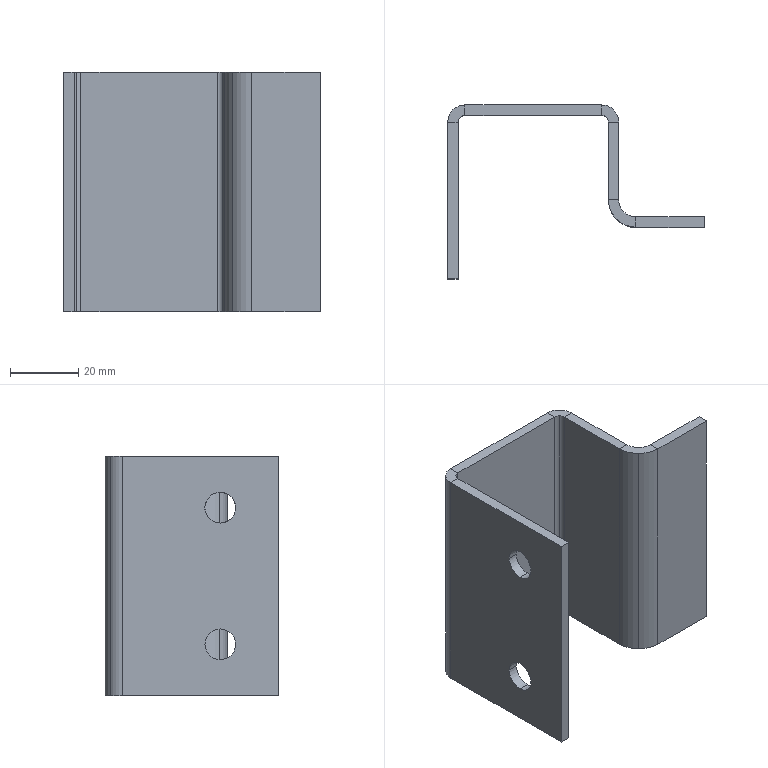Part | NX | features BREP 1 | 1 solid | 44 faces | box 75 x 50.821 x 70 mm | volume 31072 mm3 | plane 24 | cylinder 20 | commonest cylinder face diameters 9 x8 10 x6 4 x4 16 x2
STEP:
#1=CARTESIAN_POINT('',(1716.53,-660.002,420.012));
#2=VERTEX_POINT('',#1);
#3=CARTESIAN_POINT('',(1716.53,-660.002,490.012));
#4=VERTEX_POINT('',#3);
#5=CARTESIAN_POINT('',(1716.53,-660.002,455.012));
#6=DIRECTION('',(0.,0.,1.));
#7=VECTOR('',#6,1000.);
#8=LINE('',#5,#7);
#9=EDGE_CURVE('',#2,#4,#8,.T.);
#10=ORIENTED_EDGE('',*,*,#9,.T.);
#11=CARTESIAN_POINT('',(1696.53,-660.002,490.012));
#12=VERTEX_POINT('',#11);
#13=CARTESIAN_POINT('',(1706.53,-660.002,490.012));
#14=DIRECTION('',(1.,0.,0.));
#15=VECTOR('',#14,1000.);
#16=LINE('',#13,#15);
#17=EDGE_CURVE('',#12,#4,#16,.T.);
#18=ORIENTED_EDGE('',*,*,#17,.F.);
#19=CARTESIAN_POINT('',(1696.53,-660.002,420.012));
#20=VERTEX_POINT('',#19);
#21=CARTESIAN_POINT('',(1696.53,-660.002,455.012));
#22=DIRECTION('',(0.,0.,1.));
#23=VECTOR('',#22,1000.);
#24=LINE('',#21,#23);
#25=EDGE_CURVE('',#20,#12,#24,.T.);
#26=ORIENTED_EDGE('',*,*,#25,.F.);
#27=CARTESIAN_POINT('',(1706.53,-660.002,420.012));
#28=DIRECTION('',(1.,0.,0.));
#29=VECTOR('',#28,1000.);
#30=LINE('',#27,#29);
#31=EDGE_CURVE('',#20,#2,#30,.T.);
#32=ORIENTED_EDGE('',*,*,#31,.T.);
#33=EDGE_LOOP('',(#10,#18,#26,#32));
#34=FACE_BOUND('',#33,.T.);
#35=CARTESIAN_POINT('',(1691.53,-660.002,455.012));
#36=DIRECTION('',(0.,-1.,0.));
#37=DIRECTION('',(1.,0.,0.));
#38=AXIS2_PLACEMENT_3D('',#35,#36,#37);
#39=PLANE('',#38);
#40=ADVANCED_FACE('',(#34),#39,.T.);
#41=CARTESIAN_POINT('',(1696.53,-657.002,420.012));
#42=VERTEX_POINT('',#41);
#43=CARTESIAN_POINT('',(1716.53,-657.002,420.012));
#44=VERTEX_POINT('',#43);
#45=CARTESIAN_POINT('',(1706.53,-657.002,420.012));
#46=DIRECTION('',(1.,0.,0.));
#47=VECTOR('',#46,1000.);
#48=LINE('',#45,#47);
#49=EDGE_CURVE('',#42,#44,#48,.T.);
#50=ORIENTED_EDGE('',*,*,#49,.F.);
#51=CARTESIAN_POINT('',(1696.53,-657.002,490.012));
#52=VERTEX_POINT('',#51);
#53=CARTESIAN_POINT('',(1696.53,-657.002,455.012));
#54=DIRECTION('',(0.,0.,1.));
#55=VECTOR('',#54,1000.);
#56=LINE('',#53,#55);
#57=EDGE_CURVE('',#42,#52,#56,.T.);
#58=ORIENTED_EDGE('',*,*,#57,.T.);
#59=CARTESIAN_POINT('',(1716.53,-657.002,490.012));
#60=VERTEX_POINT('',#59);
#61=CARTESIAN_POINT('',(1706.53,-657.002,490.012));
#62=DIRECTION('',(1.,0.,0.));
#63=VECTOR('',#62,1000.);
#64=LINE('',#61,#63);
#65=EDGE_CURVE('',#52,#60,#64,.T.);
#66=ORIENTED_EDGE('',*,*,#65,.T.);
#67=CARTESIAN_POINT('',(1716.53,-657.002,455.012));
#68=DIRECTION('',(0.,0.,1.));
#69=VECTOR('',#68,1000.);
#70=LINE('',#67,#69);
#71=EDGE_CURVE('',#44,#60,#70,.T.);
#72=ORIENTED_EDGE('',*,*,#71,.F.);
#73=EDGE_LOOP('',(#50,#58,#66,#72));
#74=FACE_BOUND('',#73,.T.);
#75=CARTESIAN_POINT('',(1691.53,-657.002,455.012));
#76=DIRECTION('',(0.,-1.,0.));
#77=DIRECTION('',(1.,0.,0.));
#78=AXIS2_PLACEMENT_3D('',#75,#76,#77);
#79=PLANE('',#78);
#80=ADVANCED_FACE('',(#74),#79,.F.);
#81=ORIENTED_EDGE('',*,*,#9,.F.);
#82=CARTESIAN_POINT('',(1716.53,-658.502,420.012));
#83=DIRECTION('',(0.,1.,0.));
#84=VECTOR('',#83,1000.);
#85=LINE('',#82,#84);
#86=EDGE_CURVE('',#2,#44,#85,.T.);
#87=ORIENTED_EDGE('',*,*,#86,.T.);
#88=ORIENTED_EDGE('',*,*,#71,.T.);
#89=CARTESIAN_POINT('',(1716.53,-658.502,490.012));
#90=DIRECTION('',(0.,1.,0.));
#91=VECTOR('',#90,1000.);
#92=LINE('',#89,#91);
#93=EDGE_CURVE('',#4,#60,#92,.T.);
#94=ORIENTED_EDGE('',*,*,#93,.F.);
#95=EDGE_LOOP('',(#81,#87,#88,#94));
#96=FACE_BOUND('',#95,.T.);
#97=CARTESIAN_POINT('',(1716.53,-660.002,455.012));
#98=DIRECTION('',(1.,0.,0.));
#99=DIRECTION('',(0.,1.,0.));
#100=AXIS2_PLACEMENT_3D('',#97,#98,#99);
#101=PLANE('',#100);
#102=ADVANCED_FACE('',(#96),#101,.T.);
#103=ORIENTED_EDGE('',*,*,#31,.F.);
#104=CARTESIAN_POINT('',(1696.53,-658.502,420.012));
#105=DIRECTION('',(0.,-1.,0.));
#106=VECTOR('',#105,1000.);
#107=LINE('',#104,#106);
#108=EDGE_CURVE('',#42,#20,#107,.T.);
#109=ORIENTED_EDGE('',*,*,#108,.F.);
#110=ORIENTED_EDGE('',*,*,#49,.T.);
#111=ORIENTED_EDGE('',*,*,#86,.F.);
#112=EDGE_LOOP('',(#103,#109,#110,#111));
#113=FACE_BOUND('',#112,.T.);
#114=CARTESIAN_POINT('',(1706.53,-660.002,420.012));
#115=DIRECTION('',(0.,0.,1.));
#116=DIRECTION('',(1.,0.,0.));
#117=AXIS2_PLACEMENT_3D('',#114,#115,#116);
#118=PLANE('',#117);
#119=ADVANCED_FACE('',(#113),#118,.F.);
#120=CARTESIAN_POINT('',(1690.873,-657.658,420.012));
#121=VERTEX_POINT('',#120);
#122=CARTESIAN_POINT('',(1690.873,-657.658,490.012));
#123=VERTEX_POINT('',#122);
#124=CARTESIAN_POINT('',(1690.873,-657.658,455.012));
#125=DIRECTION('',(0.,0.,1.));
#126=VECTOR('',#125,1000.);
#127=LINE('',#124,#126);
#128=EDGE_CURVE('',#121,#123,#127,.T.);
#129=ORIENTED_EDGE('',*,*,#128,.F.);
#130=CARTESIAN_POINT('',(1696.53,-652.002,420.012));
#131=DIRECTION('',(0.,0.,1.));
#132=DIRECTION('',(1.,0.,0.));
#133=AXIS2_PLACEMENT_3D('',#130,#131,#132);
#134=CIRCLE('',#133,8.);
#135=EDGE_CURVE('',#121,#20,#134,.T.);
#136=ORIENTED_EDGE('',*,*,#135,.T.);
#137=ORIENTED_EDGE('',*,*,#25,.T.);
#138=CARTESIAN_POINT('',(1696.53,-652.002,490.012));
#139=DIRECTION('',(0.,0.,1.));
#140=DIRECTION('',(1.,0.,0.));
#141=AXIS2_PLACEMENT_3D('',#138,#139,#140);
#142=CIRCLE('',#141,8.);
#143=EDGE_CURVE('',#123,#12,#142,.T.);
#144=ORIENTED_EDGE('',*,*,#143,.F.);
#145=EDGE_LOOP('',(#129,#136,#137,#144));
#146=FACE_BOUND('',#145,.T.);
#147=CARTESIAN_POINT('',(1696.53,-652.002,455.012));
#148=DIRECTION('',(0.,0.,1.));
#149=DIRECTION('',(-0.7071,-0.7071,0.));
#150=AXIS2_PLACEMENT_3D('',#147,#148,#149);
#151=CYLINDRICAL_SURFACE('',#150,8.);
#152=ADVANCED_FACE('',(#146),#151,.T.);
#153=CARTESIAN_POINT('',(1691.53,-652.002,420.012));
#154=VERTEX_POINT('',#153);
#155=CARTESIAN_POINT('',(1692.995,-655.537,420.012));
#156=VERTEX_POINT('',#155);
#157=CARTESIAN_POINT('',(1696.53,-652.002,420.012));
#158=DIRECTION('',(0.,0.,1.));
#159=DIRECTION('',(1.,0.,0.));
#160=AXIS2_PLACEMENT_3D('',#157,#158,#159);
#161=CIRCLE('',#160,5.);
#162=EDGE_CURVE('',#154,#156,#161,.T.);
#163=ORIENTED_EDGE('',*,*,#162,.F.);
#164=CARTESIAN_POINT('',(1691.53,-652.002,490.012));
#165=VERTEX_POINT('',#164);
#166=CARTESIAN_POINT('',(1691.53,-652.002,455.012));
#167=DIRECTION('',(0.,0.,1.));
#168=VECTOR('',#167,1000.);
#169=LINE('',#166,#168);
#170=EDGE_CURVE('',#154,#165,#169,.T.);
#171=ORIENTED_EDGE('',*,*,#170,.T.);
#172=CARTESIAN_POINT('',(1692.995,-655.537,490.012));
#173=VERTEX_POINT('',#172);
#174=CARTESIAN_POINT('',(1696.53,-652.002,490.012));
#175=DIRECTION('',(0.,0.,1.));
#176=DIRECTION('',(1.,0.,0.));
#177=AXIS2_PLACEMENT_3D('',#174,#175,#176);
#178=CIRCLE('',#177,5.);
#179=EDGE_CURVE('',#165,#173,#178,.T.);
#180=ORIENTED_EDGE('',*,*,#179,.T.);
#181=CARTESIAN_POINT('',(1692.995,-655.537,455.012));
#182=DIRECTION('',(0.,0.,1.));
#183=VECTOR('',#182,1000.);
#184=LINE('',#181,#183);
#185=EDGE_CURVE('',#156,#173,#184,.T.);
#186=ORIENTED_EDGE('',*,*,#185,.F.);
#187=EDGE_LOOP('',(#163,#171,#180,#186));
#188=FACE_BOUND('',#187,.T.);
#189=CARTESIAN_POINT('',(1696.53,-652.002,455.012));
#190=DIRECTION('',(0.,0.,1.));
#191=DIRECTION('',(0.7071,0.7071,0.));
#192=AXIS2_PLACEMENT_3D('',#189,#190,#191);
#193=CYLINDRICAL_SURFACE('',#192,5.);
#194=ADVANCED_FACE('',(#188),#193,.F.);
#195=CARTESIAN_POINT('',(1696.53,-652.002,490.012));
#196=DIRECTION('',(0.,0.,1.));
#197=DIRECTION('',(1.,0.,0.));
#198=AXIS2_PLACEMENT_3D('',#195,#196,#197);
#199=CIRCLE('',#198,5.);
#200=EDGE_CURVE('',#173,#52,#199,.T.);
#201=ORIENTED_EDGE('',*,*,#200,.T.);
#202=ORIENTED_EDGE('',*,*,#57,.F.);
#203=CARTESIAN_POINT('',(1696.53,-652.002,420.012));
#204=DIRECTION('',(0.,0.,1.));
#205=DIRECTION('',(1.,0.,0.));
#206=AXIS2_PLACEMENT_3D('',#203,#204,#205);
#207=CIRCLE('',#206,5.);
#208=EDGE_CURVE('',#156,#42,#207,.T.);
#209=ORIENTED_EDGE('',*,*,#208,.F.);
#210=ORIENTED_EDGE('',*,*,#185,.T.);
#211=EDGE_LOOP('',(#201,#202,#209,#210));
#212=FACE_BOUND('',#211,.T.);
#213=CARTESIAN_POINT('',(1696.53,-652.002,455.012));
#214=DIRECTION('',(0.,0.,1.));
#215=DIRECTION('',(-0.7071,-0.7071,0.));
#216=AXIS2_PLACEMENT_3D('',#213,#214,#215);
#217=CYLINDRICAL_SURFACE('',#216,5.);
#218=ADVANCED_FACE('',(#212),#217,.F.);
#219=ORIENTED_EDGE('',*,*,#93,.T.);
#220=ORIENTED_EDGE('',*,*,#65,.F.);
#221=CARTESIAN_POINT('',(1696.53,-658.502,490.012));
#222=DIRECTION('',(0.,-1.,0.));
#223=VECTOR('',#222,1000.);
#224=LINE('',#221,#223);
#225=EDGE_CURVE('',#52,#12,#224,.T.);
#226=ORIENTED_EDGE('',*,*,#225,.T.);
#227=ORIENTED_EDGE('',*,*,#17,.T.);
#228=EDGE_LOOP('',(#219,#220,#226,#227));
#229=FACE_BOUND('',#228,.T.);
#230=CARTESIAN_POINT('',(1706.53,-660.002,490.012));
#231=DIRECTION('',(0.,0.,1.));
#232=DIRECTION('',(1.,0.,0.));
#233=AXIS2_PLACEMENT_3D('',#230,#231,#232);
#234=PLANE('',#233);
#235=ADVANCED_FACE('',(#229),#234,.T.);
#236=ORIENTED_EDGE('',*,*,#128,.T.);
#237=CARTESIAN_POINT('',(1688.53,-652.002,490.012));
#238=VERTEX_POINT('',#237);
#239=CARTESIAN_POINT('',(1696.53,-652.002,490.012));
#240=DIRECTION('',(0.,0.,1.));
#241=DIRECTION('',(1.,0.,0.));
#242=AXIS2_PLACEMENT_3D('',#239,#240,#241);
#243=CIRCLE('',#242,8.);
#244=EDGE_CURVE('',#238,#123,#243,.T.);
#245=ORIENTED_EDGE('',*,*,#244,.F.);
#246=CARTESIAN_POINT('',(1688.53,-652.002,420.012));
#247=VERTEX_POINT('',#246);
#248=CARTESIAN_POINT('',(1688.53,-652.002,455.012));
#249=DIRECTION('',(0.,0.,1.));
#250=VECTOR('',#249,1000.);
#251=LINE('',#248,#250);
#252=EDGE_CURVE('',#247,#238,#251,.T.);
#253=ORIENTED_EDGE('',*,*,#252,.F.);
#254=CARTESIAN_POINT('',(1696.53,-652.002,420.012));
#255=DIRECTION('',(0.,0.,1.));
#256=DIRECTION('',(1.,0.,0.));
#257=AXIS2_PLACEMENT_3D('',#254,#255,#256);
#258=CIRCLE('',#257,8.);
#259=EDGE_CURVE('',#247,#121,#258,.T.);
#260=ORIENTED_EDGE('',*,*,#259,.T.);
#261=EDGE_LOOP('',(#236,#245,#253,#260));
#262=FACE_BOUND('',#261,.T.);
#263=CARTESIAN_POINT('',(1696.53,-652.002,455.012));
#264=DIRECTION('',(0.,0.,1.));
#265=DIRECTION('',(0.7071,0.7071,0.));
#266=AXIS2_PLACEMENT_3D('',#263,#264,#265);
#267=CYLINDRICAL_SURFACE('',#266,8.);
#268=ADVANCED_FACE('',(#262),#267,.T.);
#269=ORIENTED_EDGE('',*,*,#135,.F.);
#270=ORIENTED_EDGE('',*,*,#259,.F.);
#271=CARTESIAN_POINT('',(1690.03,-652.002,420.012));
#272=DIRECTION('',(-1.,0.,0.));
#273=VECTOR('',#272,1000.);
#274=LINE('',#271,#273);
#275=EDGE_CURVE('',#154,#247,#274,.T.);
#276=ORIENTED_EDGE('',*,*,#275,.F.);
#277=ORIENTED_EDGE('',*,*,#162,.T.);
#278=ORIENTED_EDGE('',*,*,#208,.T.);
#279=ORIENTED_EDGE('',*,*,#108,.T.);
#280=EDGE_LOOP('',(#269,#270,#276,#277,#278,#279));
#281=FACE_BOUND('',#280,.T.);
#282=CARTESIAN_POINT('',(1688.53,-652.002,420.012));
#283=DIRECTION('',(0.,0.,1.));
#284=DIRECTION('',(0.3827,-0.9239,0.));
#285=AXIS2_PLACEMENT_3D('',#282,#283,#284);
#286=PLANE('',#285);
#287=ADVANCED_FACE('',(#281),#286,.F.);
#288=CARTESIAN_POINT('',(1691.53,-629.251,490.012));
#289=VERTEX_POINT('',#288);
#290=CARTESIAN_POINT('',(1691.53,-640.626,490.012));
#291=DIRECTION('',(0.,1.,0.));
#292=VECTOR('',#291,1000.);
#293=LINE('',#290,#292);
#294=EDGE_CURVE('',#165,#289,#293,.T.);
#295=ORIENTED_EDGE('',*,*,#294,.F.);
#296=ORIENTED_EDGE('',*,*,#170,.F.);
#297=CARTESIAN_POINT('',(1691.53,-629.251,420.012));
#298=VERTEX_POINT('',#297);
#299=CARTESIAN_POINT('',(1691.53,-640.626,420.012));
#300=DIRECTION('',(0.,-1.,0.));
#301=VECTOR('',#300,1000.);
#302=LINE('',#299,#301);
#303=EDGE_CURVE('',#298,#154,#302,.T.);
#304=ORIENTED_EDGE('',*,*,#303,.F.);
#305=CARTESIAN_POINT('',(1691.53,-629.251,455.012));
#306=DIRECTION('',(0.,0.,1.));
#307=VECTOR('',#306,1000.);
#308=LINE('',#305,#307);
#309=EDGE_CURVE('',#298,#289,#308,.T.);
#310=ORIENTED_EDGE('',*,*,#309,.T.);
#311=EDGE_LOOP('',(#295,#296,#304,#310));
#312=FACE_BOUND('',#311,.T.);
#313=CARTESIAN_POINT('',(1691.53,-624.251,455.012));
#314=DIRECTION('',(-1.,0.,0.));
#315=DIRECTION('',(0.,-1.,0.));
#316=AXIS2_PLACEMENT_3D('',#313,#314,#315);
#317=PLANE('',#316);
#318=ADVANCED_FACE('',(#312),#317,.F.);
#319=ORIENTED_EDGE('',*,*,#225,.F.);
#320=ORIENTED_EDGE('',*,*,#200,.F.);
#321=ORIENTED_EDGE('',*,*,#179,.F.);
#322=CARTESIAN_POINT('',(1690.03,-652.002,490.012));
#323=DIRECTION('',(-1.,0.,0.));
#324=VECTOR('',#323,1000.);
#325=LINE('',#322,#324);
#326=EDGE_CURVE('',#165,#238,#325,.T.);
#327=ORIENTED_EDGE('',*,*,#326,.T.);
#328=ORIENTED_EDGE('',*,*,#244,.T.);
#329=ORIENTED_EDGE('',*,*,#143,.T.);
#330=EDGE_LOOP('',(#319,#320,#321,#327,#328,#329));
#331=FACE_BOUND('',#330,.T.);
#332=CARTESIAN_POINT('',(1688.53,-652.002,490.012));
#333=DIRECTION('',(0.,0.,1.));
#334=DIRECTION('',(0.3827,-0.9239,0.));
#335=AXIS2_PLACEMENT_3D('',#332,#333,#334);
#336=PLANE('',#335);
#337=ADVANCED_FACE('',(#331),#336,.T.);
#338=CARTESIAN_POINT('',(1688.53,-629.251,420.012));
#339=VERTEX_POINT('',#338);
#340=CARTESIAN_POINT('',(1688.53,-629.251,490.012));
#341=VERTEX_POINT('',#340);
#342=CARTESIAN_POINT('',(1688.53,-629.251,455.012));
#343=DIRECTION('',(0.,0.,1.));
#344=VECTOR('',#343,1000.);
#345=LINE('',#342,#344);
#346=EDGE_CURVE('',#339,#341,#345,.T.);
#347=ORIENTED_EDGE('',*,*,#346,.F.);
#348=CARTESIAN_POINT('',(1688.53,-640.626,420.012));
#349=DIRECTION('',(0.,-1.,0.));
#350=VECTOR('',#349,1000.);
#351=LINE('',#348,#350);
#352=EDGE_CURVE('',#339,#247,#351,.T.);
#353=ORIENTED_EDGE('',*,*,#352,.T.);
#354=ORIENTED_EDGE('',*,*,#252,.T.);
#355=CARTESIAN_POINT('',(1688.53,-640.626,490.012));
#356=DIRECTION('',(0.,1.,0.));
#357=VECTOR('',#356,1000.);
#358=LINE('',#355,#357);
#359=EDGE_CURVE('',#238,#341,#358,.T.);
#360=ORIENTED_EDGE('',*,*,#359,.T.);
#361=EDGE_LOOP('',(#347,#353,#354,#360));
#362=FACE_BOUND('',#361,.T.);
#363=CARTESIAN_POINT('',(1688.53,-624.251,455.012));
#364=DIRECTION('',(-1.,0.,0.));
#365=DIRECTION('',(0.,-1.,0.));
#366=AXIS2_PLACEMENT_3D('',#363,#364,#365);
#367=PLANE('',#366);
#368=ADVANCED_FACE('',(#362),#367,.T.);
#369=CARTESIAN_POINT('',(1690.03,-629.251,420.012));
#370=DIRECTION('',(1.,0.,0.));
#371=VECTOR('',#370,1000.);
#372=LINE('',#369,#371);
#373=EDGE_CURVE('',#339,#298,#372,.T.);
#374=ORIENTED_EDGE('',*,*,#373,.T.);
#375=ORIENTED_EDGE('',*,*,#303,.T.);
#376=ORIENTED_EDGE('',*,*,#275,.T.);
#377=ORIENTED_EDGE('',*,*,#352,.F.);
#378=EDGE_LOOP('',(#374,#375,#376,#377));
#379=FACE_BOUND('',#378,.T.);
#380=CARTESIAN_POINT('',(1688.53,-640.626,420.012));
#381=DIRECTION('',(0.,0.,1.));
#382=DIRECTION('',(1.,0.,0.));
#383=AXIS2_PLACEMENT_3D('',#380,#381,#382);
#384=PLANE('',#383);
#385=ADVANCED_FACE('',(#379),#384,.F.);
#386=CARTESIAN_POINT('',(1690.066,-625.715,420.012));
#387=VERTEX_POINT('',#386);
#388=CARTESIAN_POINT('',(1690.066,-625.715,490.012));
#389=VERTEX_POINT('',#388);
#390=CARTESIAN_POINT('',(1690.066,-625.715,455.012));
#391=DIRECTION('',(0.,0.,1.));
#392=VECTOR('',#391,1000.);
#393=LINE('',#390,#392);
#394=EDGE_CURVE('',#387,#389,#393,.T.);
#395=ORIENTED_EDGE('',*,*,#394,.T.);
#396=CARTESIAN_POINT('',(1686.53,-629.251,490.012));
#397=DIRECTION('',(0.,0.,1.));
#398=DIRECTION('',(1.,0.,0.));
#399=AXIS2_PLACEMENT_3D('',#396,#397,#398);
#400=CIRCLE('',#399,5.);
#401=EDGE_CURVE('',#289,#389,#400,.T.);
#402=ORIENTED_EDGE('',*,*,#401,.F.);
#403=ORIENTED_EDGE('',*,*,#309,.F.);
#404=CARTESIAN_POINT('',(1686.53,-629.251,420.012));
#405=DIRECTION('',(0.,0.,1.));
#406=DIRECTION('',(1.,0.,0.));
#407=AXIS2_PLACEMENT_3D('',#404,#405,#406);
#408=CIRCLE('',#407,5.);
#409=EDGE_CURVE('',#298,#387,#408,.T.);
#410=ORIENTED_EDGE('',*,*,#409,.T.);
#411=EDGE_LOOP('',(#395,#402,#403,#410));
#412=FACE_BOUND('',#411,.T.);
#413=CARTESIAN_POINT('',(1686.53,-629.251,455.012));
#414=DIRECTION('',(0.,0.,1.));
#415=DIRECTION('',(-0.7071,-0.7071,0.));
#416=AXIS2_PLACEMENT_3D('',#413,#414,#415);
#417=CYLINDRICAL_SURFACE('',#416,5.);
#418=ADVANCED_FACE('',(#412),#417,.T.);
#419=ORIENTED_EDGE('',*,*,#359,.F.);
#420=ORIENTED_EDGE('',*,*,#326,.F.);
#421=ORIENTED_EDGE('',*,*,#294,.T.);
#422=CARTESIAN_POINT('',(1690.03,-629.251,490.012));
#423=DIRECTION('',(1.,0.,0.));
#424=VECTOR('',#423,1000.);
#425=LINE('',#422,#424);
#426=EDGE_CURVE('',#341,#289,#425,.T.);
#427=ORIENTED_EDGE('',*,*,#426,.F.);
#428=EDGE_LOOP('',(#419,#420,#421,#427));
#429=FACE_BOUND('',#428,.T.);
#430=CARTESIAN_POINT('',(1688.53,-640.626,490.012));
#431=DIRECTION('',(0.,0.,1.));
#432=DIRECTION('',(1.,0.,0.));
#433=AXIS2_PLACEMENT_3D('',#430,#431,#432);
#434=PLANE('',#433);
#435=ADVANCED_FACE('',(#429),#434,.T.);
#436=CARTESIAN_POINT('',(1687.944,-627.837,420.012));
#437=VERTEX_POINT('',#436);
#438=CARTESIAN_POINT('',(1686.53,-629.251,420.012));
#439=DIRECTION('',(0.,0.,1.));
#440=DIRECTION('',(1.,0.,0.));
#441=AXIS2_PLACEMENT_3D('',#438,#439,#440);
#442=CIRCLE('',#441,2.);
#443=EDGE_CURVE('',#339,#437,#442,.T.);
#444=ORIENTED_EDGE('',*,*,#443,.F.);
#445=ORIENTED_EDGE('',*,*,#346,.T.);
#446=CARTESIAN_POINT('',(1687.944,-627.837,490.012));
#447=VERTEX_POINT('',#446);
#448=CARTESIAN_POINT('',(1686.53,-629.251,490.012));
#449=DIRECTION('',(0.,0.,1.));
#450=DIRECTION('',(1.,0.,0.));
#451=AXIS2_PLACEMENT_3D('',#448,#449,#450);
#452=CIRCLE('',#451,2.);
#453=EDGE_CURVE('',#341,#447,#452,.T.);
#454=ORIENTED_EDGE('',*,*,#453,.T.);
#455=CARTESIAN_POINT('',(1687.944,-627.837,455.012));
#456=DIRECTION('',(0.,0.,1.));
#457=VECTOR('',#456,1000.);
#458=LINE('',#455,#457);
#459=EDGE_CURVE('',#437,#447,#458,.T.);
#460=ORIENTED_EDGE('',*,*,#459,.F.);
#461=EDGE_LOOP('',(#444,#445,#454,#460));
#462=FACE_BOUND('',#461,.T.);
#463=CARTESIAN_POINT('',(1686.53,-629.251,455.012));
#464=DIRECTION('',(0.,0.,1.));
#465=DIRECTION('',(-0.7071,-0.7071,0.));
#466=AXIS2_PLACEMENT_3D('',#463,#464,#465);
#467=CYLINDRICAL_SURFACE('',#466,2.);
#468=ADVANCED_FACE('',(#462),#467,.F.);
#469=CARTESIAN_POINT('',(1686.53,-627.251,490.012));
#470=VERTEX_POINT('',#469);
#471=CARTESIAN_POINT('',(1686.53,-629.251,490.012));
#472=DIRECTION('',(0.,0.,1.));
#473=DIRECTION('',(1.,0.,0.));
#474=AXIS2_PLACEMENT_3D('',#471,#472,#473);
#475=CIRCLE('',#474,2.);
#476=EDGE_CURVE('',#447,#470,#475,.T.);
#477=ORIENTED_EDGE('',*,*,#476,.T.);
#478=CARTESIAN_POINT('',(1686.53,-627.251,420.012));
#479=VERTEX_POINT('',#478);
#480=CARTESIAN_POINT('',(1686.53,-627.251,455.012));
#481=DIRECTION('',(0.,0.,1.));
#482=VECTOR('',#481,1000.);
#483=LINE('',#480,#482);
#484=EDGE_CURVE('',#479,#470,#483,.T.);
#485=ORIENTED_EDGE('',*,*,#484,.F.);
#486=CARTESIAN_POINT('',(1686.53,-629.251,420.012));
#487=DIRECTION('',(0.,0.,1.));
#488=DIRECTION('',(1.,0.,0.));
#489=AXIS2_PLACEMENT_3D('',#486,#487,#488);
#490=CIRCLE('',#489,2.);
#491=EDGE_CURVE('',#437,#479,#490,.T.);
#492=ORIENTED_EDGE('',*,*,#491,.F.);
#493=ORIENTED_EDGE('',*,*,#459,.T.);
#494=EDGE_LOOP('',(#477,#485,#492,#493));
#495=FACE_BOUND('',#494,.T.);
#496=CARTESIAN_POINT('',(1686.53,-629.251,455.012));
#497=DIRECTION('',(0.,0.,1.));
#498=DIRECTION('',(0.7071,0.7071,0.));
#499=AXIS2_PLACEMENT_3D('',#496,#497,#498);
#500=CYLINDRICAL_SURFACE('',#499,2.);
#501=ADVANCED_FACE('',(#495),#500,.F.);
#502=CARTESIAN_POINT('',(1686.53,-624.251,420.012));
#503=VERTEX_POINT('',#502);
#504=CARTESIAN_POINT('',(1686.53,-625.751,420.012));
#505=DIRECTION('',(0.,-1.,0.));
#506=VECTOR('',#505,1000.);
#507=LINE('',#504,#506);
#508=EDGE_CURVE('',#503,#479,#507,.T.);
#509=ORIENTED_EDGE('',*,*,#508,.F.);
#510=CARTESIAN_POINT('',(1686.53,-629.251,420.012));
#511=DIRECTION('',(0.,0.,1.));
#512=DIRECTION('',(1.,0.,0.));
#513=AXIS2_PLACEMENT_3D('',#510,#511,#512);
#514=CIRCLE('',#513,5.);
#515=EDGE_CURVE('',#387,#503,#514,.T.);
#516=ORIENTED_EDGE('',*,*,#515,.F.);
#517=ORIENTED_EDGE('',*,*,#409,.F.);
#518=ORIENTED_EDGE('',*,*,#373,.F.);
#519=ORIENTED_EDGE('',*,*,#443,.T.);
#520=ORIENTED_EDGE('',*,*,#491,.T.);
#521=EDGE_LOOP('',(#509,#516,#517,#518,#519,#520));
#522=FACE_BOUND('',#521,.T.);
#523=CARTESIAN_POINT('',(1688.53,-629.251,420.012));
#524=DIRECTION('',(0.,0.,1.));
#525=DIRECTION('',(-0.3827,0.9239,0.));
#526=AXIS2_PLACEMENT_3D('',#523,#524,#525);
#527=PLANE('',#526);
#528=ADVANCED_FACE('',(#522),#527,.F.);
#529=ORIENTED_EDGE('',*,*,#394,.F.);
#530=ORIENTED_EDGE('',*,*,#515,.T.);
#531=CARTESIAN_POINT('',(1686.53,-624.251,490.012));
#532=VERTEX_POINT('',#531);
#533=CARTESIAN_POINT('',(1686.53,-624.251,455.012));
#534=DIRECTION('',(0.,0.,1.));
#535=VECTOR('',#534,1000.);
#536=LINE('',#533,#535);
#537=EDGE_CURVE('',#503,#532,#536,.T.);
#538=ORIENTED_EDGE('',*,*,#537,.T.);
#539=CARTESIAN_POINT('',(1686.53,-629.251,490.012));
#540=DIRECTION('',(0.,0.,1.));
#541=DIRECTION('',(1.,0.,0.));
#542=AXIS2_PLACEMENT_3D('',#539,#540,#541);
#543=CIRCLE('',#542,5.);
#544=EDGE_CURVE('',#389,#532,#543,.T.);
#545=ORIENTED_EDGE('',*,*,#544,.F.);
#546=EDGE_LOOP('',(#529,#530,#538,#545));
#547=FACE_BOUND('',#546,.T.);
#548=CARTESIAN_POINT('',(1686.53,-629.251,455.012));
#549=DIRECTION('',(0.,0.,1.));
#550=DIRECTION('',(0.7071,0.7071,0.));
#551=AXIS2_PLACEMENT_3D('',#548,#549,#550);
#552=CYLINDRICAL_SURFACE('',#551,5.);
#553=ADVANCED_FACE('',(#547),#552,.T.);
#554=ORIENTED_EDGE('',*,*,#476,.F.);
#555=ORIENTED_EDGE('',*,*,#453,.F.);
#556=ORIENTED_EDGE('',*,*,#426,.T.);
#557=ORIENTED_EDGE('',*,*,#401,.T.);
#558=ORIENTED_EDGE('',*,*,#544,.T.);
#559=CARTESIAN_POINT('',(1686.53,-625.751,490.012));
#560=DIRECTION('',(0.,-1.,0.));
#561=VECTOR('',#560,1000.);
#562=LINE('',#559,#561);
#563=EDGE_CURVE('',#532,#470,#562,.T.);
#564=ORIENTED_EDGE('',*,*,#563,.T.);
#565=EDGE_LOOP('',(#554,#555,#556,#557,#558,#564));
#566=FACE_BOUND('',#565,.T.);
#567=CARTESIAN_POINT('',(1688.53,-629.251,490.012));
#568=DIRECTION('',(0.,0.,1.));
#569=DIRECTION('',(-0.3827,0.9239,0.));
#570=AXIS2_PLACEMENT_3D('',#567,#568,#569);
#571=PLANE('',#570);
#572=ADVANCED_FACE('',(#566),#571,.T.);
#573=CARTESIAN_POINT('',(1646.53,-627.251,420.012));
#574=VERTEX_POINT('',#573);
#575=CARTESIAN_POINT('',(1646.53,-627.251,490.012));
#576=VERTEX_POINT('',#575);
#577=CARTESIAN_POINT('',(1646.53,-627.251,455.012));
#578=DIRECTION('',(0.,0.,1.));
#579=VECTOR('',#578,1000.);
#580=LINE('',#577,#579);
#581=EDGE_CURVE('',#574,#576,#580,.T.);
#582=ORIENTED_EDGE('',*,*,#581,.F.);
#583=CARTESIAN_POINT('',(1666.53,-627.251,420.012));
#584=DIRECTION('',(1.,0.,0.));
#585=VECTOR('',#584,1000.);
#586=LINE('',#583,#585);
#587=EDGE_CURVE('',#574,#479,#586,.T.);
#588=ORIENTED_EDGE('',*,*,#587,.T.);
#589=ORIENTED_EDGE('',*,*,#484,.T.);
#590=CARTESIAN_POINT('',(1666.53,-627.251,490.012));
#591=DIRECTION('',(1.,0.,0.));
#592=VECTOR('',#591,1000.);
#593=LINE('',#590,#592);
#594=EDGE_CURVE('',#576,#470,#593,.T.);
#595=ORIENTED_EDGE('',*,*,#594,.F.);
#596=EDGE_LOOP('',(#582,#588,#589,#595));
#597=FACE_BOUND('',#596,.T.);
#598=CARTESIAN_POINT('',(1641.53,-627.251,455.012));
#599=DIRECTION('',(0.,-1.,0.));
#600=DIRECTION('',(1.,0.,0.));
#601=AXIS2_PLACEMENT_3D('',#598,#599,#600);
#602=PLANE('',#601);
#603=ADVANCED_FACE('',(#597),#602,.T.);
#604=CARTESIAN_POINT('',(1646.53,-624.251,420.012));
#605=VERTEX_POINT('',#604);
#606=CARTESIAN_POINT('',(1646.53,-625.751,420.012));
#607=DIRECTION('',(0.,1.,0.));
#608=VECTOR('',#607,1000.);
#609=LINE('',#606,#608);
#610=EDGE_CURVE('',#574,#605,#609,.T.);
#611=ORIENTED_EDGE('',*,*,#610,.T.);
#612=CARTESIAN_POINT('',(1666.53,-624.251,420.012));
#613=DIRECTION('',(1.,0.,0.));
#614=VECTOR('',#613,1000.);
#615=LINE('',#612,#614);
#616=EDGE_CURVE('',#605,#503,#615,.T.);
#617=ORIENTED_EDGE('',*,*,#616,.T.);
#618=ORIENTED_EDGE('',*,*,#508,.T.);
#619=ORIENTED_EDGE('',*,*,#587,.F.);
#620=EDGE_LOOP('',(#611,#617,#618,#619));
#621=FACE_BOUND('',#620,.T.);
#622=CARTESIAN_POINT('',(1666.53,-627.251,420.012));
#623=DIRECTION('',(0.,0.,1.));
#624=DIRECTION('',(1.,0.,0.));
#625=AXIS2_PLACEMENT_3D('',#622,#623,#624);
#626=PLANE('',#625);
#627=ADVANCED_FACE('',(#621),#626,.F.);
#628=CARTESIAN_POINT('',(1646.53,-624.251,490.012));
#629=VERTEX_POINT('',#628);
#630=CARTESIAN_POINT('',(1666.53,-624.251,490.012));
#631=DIRECTION('',(1.,0.,0.));
#632=VECTOR('',#631,1000.);
#633=LINE('',#630,#632);
#634=EDGE_CURVE('',#629,#532,#633,.T.);
#635=ORIENTED_EDGE('',*,*,#634,.T.);
#636=ORIENTED_EDGE('',*,*,#537,.F.);
#637=ORIENTED_EDGE('',*,*,#616,.F.);
#638=CARTESIAN_POINT('',(1646.53,-624.251,455.012));
#639=DIRECTION('',(0.,0.,1.));
#640=VECTOR('',#639,1000.);
#641=LINE('',#638,#640);
#642=EDGE_CURVE('',#605,#629,#641,.T.);
#643=ORIENTED_EDGE('',*,*,#642,.T.);
#644=EDGE_LOOP('',(#635,#636,#637,#643));
#645=FACE_BOUND('',#644,.T.);
#646=CARTESIAN_POINT('',(1641.53,-624.251,455.012));
#647=DIRECTION('',(0.,-1.,0.));
#648=DIRECTION('',(1.,0.,0.));
#649=AXIS2_PLACEMENT_3D('',#646,#647,#648);
#650=PLANE('',#649);
#651=ADVANCED_FACE('',(#645),#650,.F.);
#652=ORIENTED_EDGE('',*,*,#594,.T.);
#653=ORIENTED_EDGE('',*,*,#563,.F.);
#654=ORIENTED_EDGE('',*,*,#634,.F.);
#655=CARTESIAN_POINT('',(1646.53,-625.751,490.012));
#656=DIRECTION('',(0.,1.,0.));
#657=VECTOR('',#656,1000.);
#658=LINE('',#655,#657);
#659=EDGE_CURVE('',#576,#629,#658,.T.);
#660=ORIENTED_EDGE('',*,*,#659,.F.);
#661=EDGE_LOOP('',(#652,#653,#654,#660));
#662=FACE_BOUND('',#661,.T.);
#663=CARTESIAN_POINT('',(1666.53,-627.251,490.012));
#664=DIRECTION('',(0.,0.,1.));
#665=DIRECTION('',(1.,0.,0.));
#666=AXIS2_PLACEMENT_3D('',#663,#664,#665);
#667=PLANE('',#666);
#668=ADVANCED_FACE('',(#662),#667,.T.);
#669=CARTESIAN_POINT('',(1645.116,-627.837,420.012));
#670=VERTEX_POINT('',#669);
#671=CARTESIAN_POINT('',(1646.53,-629.251,420.012));
#672=DIRECTION('',(0.,0.,1.));
#673=DIRECTION('',(1.,0.,0.));
#674=AXIS2_PLACEMENT_3D('',#671,#672,#673);
#675=CIRCLE('',#674,2.);
#676=EDGE_CURVE('',#574,#670,#675,.T.);
#677=ORIENTED_EDGE('',*,*,#676,.F.);
#678=ORIENTED_EDGE('',*,*,#581,.T.);
#679=CARTESIAN_POINT('',(1645.116,-627.837,490.012));
#680=VERTEX_POINT('',#679);
#681=CARTESIAN_POINT('',(1646.53,-629.251,490.012));
#682=DIRECTION('',(0.,0.,1.));
#683=DIRECTION('',(1.,0.,0.));
#684=AXIS2_PLACEMENT_3D('',#681,#682,#683);
#685=CIRCLE('',#684,2.);
#686=EDGE_CURVE('',#576,#680,#685,.T.);
#687=ORIENTED_EDGE('',*,*,#686,.T.);
#688=CARTESIAN_POINT('',(1645.116,-627.837,455.012));
#689=DIRECTION('',(0.,0.,1.));
#690=VECTOR('',#689,1000.);
#691=LINE('',#688,#690);
#692=EDGE_CURVE('',#670,#680,#691,.T.);
#693=ORIENTED_EDGE('',*,*,#692,.F.);
#694=EDGE_LOOP('',(#677,#678,#687,#693));
#695=FACE_BOUND('',#694,.T.);
#696=CARTESIAN_POINT('',(1646.53,-629.251,455.012));
#697=DIRECTION('',(0.,0.,1.));
#698=DIRECTION('',(0.7071,-0.7071,0.));
#699=AXIS2_PLACEMENT_3D('',#696,#697,#698);
#700=CYLINDRICAL_SURFACE('',#699,2.);
#701=ADVANCED_FACE('',(#695),#700,.F.);
#702=CARTESIAN_POINT('',(1641.53,-629.251,420.012));
#703=VERTEX_POINT('',#702);
#704=CARTESIAN_POINT('',(1644.53,-629.251,420.012));
#705=VERTEX_POINT('',#704);
#706=CARTESIAN_POINT('',(1643.03,-629.251,420.012));
#707=DIRECTION('',(1.,0.,0.));
#708=VECTOR('',#707,1000.);
#709=LINE('',#706,#708);
#710=EDGE_CURVE('',#703,#705,#709,.T.);
#711=ORIENTED_EDGE('',*,*,#710,.F.);
#712=CARTESIAN_POINT('',(1642.995,-625.715,420.012));
#713=VERTEX_POINT('',#712);
#714=CARTESIAN_POINT('',(1646.53,-629.251,420.012));
#715=DIRECTION('',(0.,0.,1.));
#716=DIRECTION('',(1.,0.,0.));
#717=AXIS2_PLACEMENT_3D('',#714,#715,#716);
#718=CIRCLE('',#717,5.);
#719=EDGE_CURVE('',#713,#703,#718,.T.);
#720=ORIENTED_EDGE('',*,*,#719,.F.);
#721=CARTESIAN_POINT('',(1646.53,-629.251,420.012));
#722=DIRECTION('',(0.,0.,1.));
#723=DIRECTION('',(1.,0.,0.));
#724=AXIS2_PLACEMENT_3D('',#721,#722,#723);
#725=CIRCLE('',#724,5.);
#726=EDGE_CURVE('',#605,#713,#725,.T.);
#727=ORIENTED_EDGE('',*,*,#726,.F.);
#728=ORIENTED_EDGE('',*,*,#610,.F.);
#729=ORIENTED_EDGE('',*,*,#676,.T.);
#730=CARTESIAN_POINT('',(1646.53,-629.251,420.012));
#731=DIRECTION('',(0.,0.,1.));
#732=DIRECTION('',(1.,0.,0.));
#733=AXIS2_PLACEMENT_3D('',#730,#731,#732);
#734=CIRCLE('',#733,2.);
#735=EDGE_CURVE('',#670,#705,#734,.T.);
#736=ORIENTED_EDGE('',*,*,#735,.T.);
#737=EDGE_LOOP('',(#711,#720,#727,#728,#729,#736));
#738=FACE_BOUND('',#737,.T.);
#739=CARTESIAN_POINT('',(1646.53,-627.251,420.012));
#740=DIRECTION('',(0.,0.,1.));
#741=DIRECTION('',(-0.9239,-0.3827,0.));
#742=AXIS2_PLACEMENT_3D('',#739,#740,#741);
#743=PLANE('',#742);
#744=ADVANCED_FACE('',(#738),#743,.F.);
#745=CARTESIAN_POINT('',(1642.995,-625.715,490.012));
#746=VERTEX_POINT('',#745);
#747=CARTESIAN_POINT('',(1642.995,-625.715,455.012));
#748=DIRECTION('',(0.,0.,1.));
#749=VECTOR('',#748,1000.);
#750=LINE('',#747,#749);
#751=EDGE_CURVE('',#713,#746,#750,.T.);
#752=ORIENTED_EDGE('',*,*,#751,.T.);
#753=CARTESIAN_POINT('',(1646.53,-629.251,490.012));
#754=DIRECTION('',(0.,0.,1.));
#755=DIRECTION('',(1.,0.,0.));
#756=AXIS2_PLACEMENT_3D('',#753,#754,#755);
#757=CIRCLE('',#756,5.);
#758=EDGE_CURVE('',#629,#746,#757,.T.);
#759=ORIENTED_EDGE('',*,*,#758,.F.);
#760=ORIENTED_EDGE('',*,*,#642,.F.);
#761=ORIENTED_EDGE('',*,*,#726,.T.);
#762=EDGE_LOOP('',(#752,#759,#760,#761));
#763=FACE_BOUND('',#762,.T.);
#764=CARTESIAN_POINT('',(1646.53,-629.251,455.012));
#765=DIRECTION('',(0.,0.,1.));
#766=DIRECTION('',(0.7071,-0.7071,0.));
#767=AXIS2_PLACEMENT_3D('',#764,#765,#766);
#768=CYLINDRICAL_SURFACE('',#767,5.);
#769=ADVANCED_FACE('',(#763),#768,.T.);
#770=CARTESIAN_POINT('',(1644.53,-629.251,490.012));
#771=VERTEX_POINT('',#770);
#772=CARTESIAN_POINT('',(1646.53,-629.251,490.012));
#773=DIRECTION('',(0.,0.,1.));
#774=DIRECTION('',(1.,0.,0.));
#775=AXIS2_PLACEMENT_3D('',#772,#773,#774);
#776=CIRCLE('',#775,2.);
#777=EDGE_CURVE('',#680,#771,#776,.T.);
#778=ORIENTED_EDGE('',*,*,#777,.F.);
#779=ORIENTED_EDGE('',*,*,#686,.F.);
#780=ORIENTED_EDGE('',*,*,#659,.T.);
#781=ORIENTED_EDGE('',*,*,#758,.T.);
#782=CARTESIAN_POINT('',(1641.53,-629.251,490.012));
#783=VERTEX_POINT('',#782);
#784=CARTESIAN_POINT('',(1646.53,-629.251,490.012));
#785=DIRECTION('',(0.,0.,1.));
#786=DIRECTION('',(1.,0.,0.));
#787=AXIS2_PLACEMENT_3D('',#784,#785,#786);
#788=CIRCLE('',#787,5.);
#789=EDGE_CURVE('',#746,#783,#788,.T.);
#790=ORIENTED_EDGE('',*,*,#789,.T.);
#791=CARTESIAN_POINT('',(1643.03,-629.251,490.012));
#792=DIRECTION('',(1.,0.,0.));
#793=VECTOR('',#792,1000.);
#794=LINE('',#791,#793);
#795=EDGE_CURVE('',#783,#771,#794,.T.);
#796=ORIENTED_EDGE('',*,*,#795,.T.);
#797=EDGE_LOOP('',(#778,#779,#780,#781,#790,#796));
#798=FACE_BOUND('',#797,.T.);
#799=CARTESIAN_POINT('',(1646.53,-627.251,490.012));
#800=DIRECTION('',(0.,0.,1.));
#801=DIRECTION('',(-0.9239,-0.3827,0.));
#802=AXIS2_PLACEMENT_3D('',#799,#800,#801);
#803=PLANE('',#802);
#804=ADVANCED_FACE('',(#798),#803,.T.);
#805=ORIENTED_EDGE('',*,*,#777,.T.);
#806=CARTESIAN_POINT('',(1644.53,-629.251,455.012));
#807=DIRECTION('',(0.,0.,1.));
#808=VECTOR('',#807,1000.);
#809=LINE('',#806,#808);
#810=EDGE_CURVE('',#705,#771,#809,.T.);
#811=ORIENTED_EDGE('',*,*,#810,.F.);
#812=ORIENTED_EDGE('',*,*,#735,.F.);
#813=ORIENTED_EDGE('',*,*,#692,.T.);
#814=EDGE_LOOP('',(#805,#811,#812,#813));
#815=FACE_BOUND('',#814,.T.);
#816=CARTESIAN_POINT('',(1646.53,-629.251,455.012));
#817=DIRECTION('',(0.,0.,1.));
#818=DIRECTION('',(-0.7071,0.7071,0.));
#819=AXIS2_PLACEMENT_3D('',#816,#817,#818);
#820=CYLINDRICAL_SURFACE('',#819,2.);
#821=ADVANCED_FACE('',(#815),#820,.F.);
#822=CARTESIAN_POINT('',(1641.53,-657.927,430.512));
#823=VERTEX_POINT('',#822);
#824=CARTESIAN_POINT('',(1641.53,-653.427,435.012));
#825=VERTEX_POINT('',#824);
#826=CARTESIAN_POINT('',(1641.53,-657.927,435.012));
#827=DIRECTION('',(1.,0.,0.));
#828=DIRECTION('',(0.,0.,-1.));
#829=AXIS2_PLACEMENT_3D('',#826,#827,#828);
#830=CIRCLE('',#829,4.5);
#831=EDGE_CURVE('',#823,#825,#830,.T.);
#832=ORIENTED_EDGE('',*,*,#831,.F.);
#833=CARTESIAN_POINT('',(1644.53,-657.927,430.512));
#834=VERTEX_POINT('',#833);
#835=CARTESIAN_POINT('',(1644.53,-657.927,430.512));
#836=DIRECTION('',(1.,0.,0.));
#837=VECTOR('',#836,1000.);
#838=LINE('',#835,#837);
#839=EDGE_CURVE('',#823,#834,#838,.T.);
#840=ORIENTED_EDGE('',*,*,#839,.T.);
#841=CARTESIAN_POINT('',(1644.53,-653.427,435.012));
#842=VERTEX_POINT('',#841);
#843=CARTESIAN_POINT('',(1644.53,-657.927,435.012));
#844=DIRECTION('',(1.,0.,0.));
#845=DIRECTION('',(0.,0.,-1.));
#846=AXIS2_PLACEMENT_3D('',#843,#844,#845);
#847=CIRCLE('',#846,4.5);
#848=EDGE_CURVE('',#834,#842,#847,.T.);
#849=ORIENTED_EDGE('',*,*,#848,.T.);
#850=CARTESIAN_POINT('',(1644.53,-653.427,435.012));
#851=DIRECTION('',(1.,0.,0.));
#852=VECTOR('',#851,1000.);
#853=LINE('',#850,#852);
#854=EDGE_CURVE('',#825,#842,#853,.T.);
#855=ORIENTED_EDGE('',*,*,#854,.F.);
#856=EDGE_LOOP('',(#832,#840,#849,#855));
#857=FACE_BOUND('',#856,.T.);
#858=CARTESIAN_POINT('',(1644.53,-657.927,435.012));
#859=DIRECTION('',(1.,0.,0.));
#860=DIRECTION('',(0.,-1.,0.));
#861=AXIS2_PLACEMENT_3D('',#858,#859,#860);
#862=CYLINDRICAL_SURFACE('',#861,4.5);
#863=ADVANCED_FACE('',(#857),#862,.F.);
#864=CARTESIAN_POINT('',(1644.53,-662.426,475.012));
#865=VERTEX_POINT('',#864);
#866=CARTESIAN_POINT('',(1644.53,-657.926,470.512));
#867=VERTEX_POINT('',#866);
#868=CARTESIAN_POINT('',(1644.53,-657.926,475.012));
#869=DIRECTION('',(1.,0.,0.));
#870=DIRECTION('',(0.,0.,-1.));
#871=AXIS2_PLACEMENT_3D('',#868,#869,#870);
#872=CIRCLE('',#871,4.5);
#873=EDGE_CURVE('',#865,#867,#872,.T.);
#874=ORIENTED_EDGE('',*,*,#873,.T.);
#875=CARTESIAN_POINT('',(1641.53,-657.926,470.512));
#876=VERTEX_POINT('',#875);
#877=CARTESIAN_POINT('',(1644.53,-657.926,470.512));
#878=DIRECTION('',(1.,0.,0.));
#879=VECTOR('',#878,1000.);
#880=LINE('',#877,#879);
#881=EDGE_CURVE('',#876,#867,#880,.T.);
#882=ORIENTED_EDGE('',*,*,#881,.F.);
#883=CARTESIAN_POINT('',(1641.53,-662.426,475.012));
#884=VERTEX_POINT('',#883);
#885=CARTESIAN_POINT('',(1641.53,-662.426,475.012));
#886=CARTESIAN_POINT('',(1641.53,-662.426,473.831));
#887=CARTESIAN_POINT('',(1641.53,-661.449,471.489));
#888=CARTESIAN_POINT('',(1641.53,-659.109,470.512));
#889=CARTESIAN_POINT('',(1641.53,-657.926,470.512));
#890=B_SPLINE_CURVE_WITH_KNOTS('',3,(#885,#886,#887,#888,#889),.UNSPECIFIED.,.F.,.F.,(4,1,4),(0.,0.5,1.),.UNSPECIFIED.);
#891=EDGE_CURVE('',#884,#876,#890,.T.);
#892=ORIENTED_EDGE('',*,*,#891,.F.);
#893=CARTESIAN_POINT('',(1644.53,-662.426,475.012));
#894=DIRECTION('',(1.,0.,0.));
#895=VECTOR('',#894,1000.);
#896=LINE('',#893,#895);
#897=EDGE_CURVE('',#884,#865,#896,.T.);
#898=ORIENTED_EDGE('',*,*,#897,.T.);
#899=EDGE_LOOP('',(#874,#882,#892,#898));
#900=FACE_BOUND('',#899,.T.);
#901=CARTESIAN_POINT('',(1644.53,-657.926,475.012));
#902=DIRECTION('',(1.,0.,0.));
#903=DIRECTION('',(0.,-1.,0.));
#904=AXIS2_PLACEMENT_3D('',#901,#902,#903);
#905=CYLINDRICAL_SURFACE('',#904,4.5);
#906=ADVANCED_FACE('',(#900),#905,.F.);
#907=CARTESIAN_POINT('',(1641.53,-657.926,479.512));
#908=VERTEX_POINT('',#907);
#909=CARTESIAN_POINT('',(1641.53,-657.926,479.512));
#910=CARTESIAN_POINT('',(1641.53,-659.108,479.512));
#911=CARTESIAN_POINT('',(1641.53,-661.45,478.535));
#912=CARTESIAN_POINT('',(1641.53,-662.426,476.195));
#913=CARTESIAN_POINT('',(1641.53,-662.426,475.012));
#914=B_SPLINE_CURVE_WITH_KNOTS('',3,(#909,#910,#911,#912,#913),.UNSPECIFIED.,.F.,.F.,(4,1,4),(0.,0.5,1.),.UNSPECIFIED.);
#915=EDGE_CURVE('',#908,#884,#914,.T.);
#916=ORIENTED_EDGE('',*,*,#915,.F.);
#917=CARTESIAN_POINT('',(1644.53,-657.926,479.512));
#918=VERTEX_POINT('',#917);
#919=CARTESIAN_POINT('',(1644.53,-657.926,479.512));
#920=DIRECTION('',(1.,0.,0.));
#921=VECTOR('',#920,1000.);
#922=LINE('',#919,#921);
#923=EDGE_CURVE('',#908,#918,#922,.T.);
#924=ORIENTED_EDGE('',*,*,#923,.T.);
#925=CARTESIAN_POINT('',(1644.53,-657.926,475.012));
#926=DIRECTION('',(1.,0.,0.));
#927=DIRECTION('',(0.,0.,-1.));
#928=AXIS2_PLACEMENT_3D('',#925,#926,#927);
#929=CIRCLE('',#928,4.5);
#930=EDGE_CURVE('',#918,#865,#929,.T.);
#931=ORIENTED_EDGE('',*,*,#930,.T.);
#932=ORIENTED_EDGE('',*,*,#897,.F.);
#933=EDGE_LOOP('',(#916,#924,#931,#932));
#934=FACE_BOUND('',#933,.T.);
#935=CARTESIAN_POINT('',(1644.53,-657.926,475.012));
#936=DIRECTION('',(1.,0.,0.));
#937=DIRECTION('',(0.,1.,0.));
#938=AXIS2_PLACEMENT_3D('',#935,#936,#937);
#939=CYLINDRICAL_SURFACE('',#938,4.5);
#940=ADVANCED_FACE('',(#934),#939,.F.);
#941=CARTESIAN_POINT('',(1644.53,-653.426,475.012));
#942=VERTEX_POINT('',#941);
#943=CARTESIAN_POINT('',(1644.53,-657.926,475.012));
#944=DIRECTION('',(1.,0.,0.));
#945=DIRECTION('',(0.,0.,-1.));
#946=AXIS2_PLACEMENT_3D('',#943,#944,#945);
#947=CIRCLE('',#946,4.5);
#948=EDGE_CURVE('',#942,#918,#947,.T.);
#949=ORIENTED_EDGE('',*,*,#948,.T.);
#950=ORIENTED_EDGE('',*,*,#923,.F.);
#951=CARTESIAN_POINT('',(1641.53,-653.426,475.012));
#952=VERTEX_POINT('',#951);
#953=CARTESIAN_POINT('',(1641.53,-653.426,475.012));
#954=CARTESIAN_POINT('',(1641.53,-653.426,476.193));
#955=CARTESIAN_POINT('',(1641.53,-654.404,478.535));
#956=CARTESIAN_POINT('',(1641.53,-656.744,479.512));
#957=CARTESIAN_POINT('',(1641.53,-657.926,479.512));
#958=B_SPLINE_CURVE_WITH_KNOTS('',3,(#953,#954,#955,#956,#957),.UNSPECIFIED.,.F.,.F.,(4,1,4),(0.,0.5,1.),.UNSPECIFIED.);
#959=EDGE_CURVE('',#952,#908,#958,.T.);
#960=ORIENTED_EDGE('',*,*,#959,.F.);
#961=CARTESIAN_POINT('',(1644.53,-653.426,475.012));
#962=DIRECTION('',(1.,0.,0.));
#963=VECTOR('',#962,1000.);
#964=LINE('',#961,#963);
#965=EDGE_CURVE('',#952,#942,#964,.T.);
#966=ORIENTED_EDGE('',*,*,#965,.T.);
#967=EDGE_LOOP('',(#949,#950,#960,#966));
#968=FACE_BOUND('',#967,.T.);
#969=CARTESIAN_POINT('',(1644.53,-657.926,475.012));
#970=DIRECTION('',(1.,0.,0.));
#971=DIRECTION('',(0.,1.,0.));
#972=AXIS2_PLACEMENT_3D('',#969,#970,#971);
#973=CYLINDRICAL_SURFACE('',#972,4.5);
#974=ADVANCED_FACE('',(#968),#973,.F.);
#975=CARTESIAN_POINT('',(1641.53,-657.926,470.512));
#976=CARTESIAN_POINT('',(1641.53,-656.745,470.512));
#977=CARTESIAN_POINT('',(1641.53,-654.403,471.489));
#978=CARTESIAN_POINT('',(1641.53,-653.426,473.829));
#979=CARTESIAN_POINT('',(1641.53,-653.426,475.012));
#980=B_SPLINE_CURVE_WITH_KNOTS('',3,(#975,#976,#977,#978,#979),.UNSPECIFIED.,.F.,.F.,(4,1,4),(0.,0.5,1.),.UNSPECIFIED.);
#981=EDGE_CURVE('',#876,#952,#980,.T.);
#982=ORIENTED_EDGE('',*,*,#981,.F.);
#983=ORIENTED_EDGE('',*,*,#881,.T.);
#984=CARTESIAN_POINT('',(1644.53,-657.926,475.012));
#985=DIRECTION('',(1.,0.,0.));
#986=DIRECTION('',(0.,0.,-1.));
#987=AXIS2_PLACEMENT_3D('',#984,#985,#986);
#988=CIRCLE('',#987,4.5);
#989=EDGE_CURVE('',#867,#942,#988,.T.);
#990=ORIENTED_EDGE('',*,*,#989,.T.);
#991=ORIENTED_EDGE('',*,*,#965,.F.);
#992=EDGE_LOOP('',(#982,#983,#990,#991));
#993=FACE_BOUND('',#992,.T.);
#994=CARTESIAN_POINT('',(1644.53,-657.926,475.012));
#995=DIRECTION('',(1.,0.,0.));
#996=DIRECTION('',(0.,-1.,0.));
#997=AXIS2_PLACEMENT_3D('',#994,#995,#996);
#998=CYLINDRICAL_SURFACE('',#997,4.5);
#999=ADVANCED_FACE('',(#993),#998,.F.);
#1000=CARTESIAN_POINT('',(1641.53,-675.072,420.012));
#1001=VERTEX_POINT('',#1000);
#1002=CARTESIAN_POINT('',(1644.53,-675.072,420.012));
#1003=VERTEX_POINT('',#1002);
#1004=CARTESIAN_POINT('',(1643.03,-675.072,420.012));
#1005=DIRECTION('',(1.,0.,0.));
#1006=VECTOR('',#1005,1000.);
#1007=LINE('',#1004,#1006);
#1008=EDGE_CURVE('',#1001,#1003,#1007,.T.);
#1009=ORIENTED_EDGE('',*,*,#1008,.F.);
#1010=CARTESIAN_POINT('',(1641.53,-652.161,420.012));
#1011=DIRECTION('',(0.,1.,0.));
#1012=VECTOR('',#1011,1000.);
#1013=LINE('',#1010,#1012);
#1014=EDGE_CURVE('',#1001,#703,#1013,.T.);
#1015=ORIENTED_EDGE('',*,*,#1014,.T.);
#1016=ORIENTED_EDGE('',*,*,#710,.T.);
#1017=CARTESIAN_POINT('',(1644.53,-652.161,420.012));
#1018=DIRECTION('',(0.,1.,0.));
#1019=VECTOR('',#1018,1000.);
#1020=LINE('',#1017,#1019);
#1021=EDGE_CURVE('',#1003,#705,#1020,.T.);
#1022=ORIENTED_EDGE('',*,*,#1021,.F.);
#1023=EDGE_LOOP('',(#1009,#1015,#1016,#1022));
#1024=FACE_BOUND('',#1023,.T.);
#1025=CARTESIAN_POINT('',(1644.53,-652.161,420.012));
#1026=DIRECTION('',(0.,0.,1.));
#1027=DIRECTION('',(1.,0.,0.));
#1028=AXIS2_PLACEMENT_3D('',#1025,#1026,#1027);
#1029=PLANE('',#1028);
#1030=ADVANCED_FACE('',(#1024),#1029,.F.);
#1031=ORIENTED_EDGE('',*,*,#751,.F.);
#1032=ORIENTED_EDGE('',*,*,#719,.T.);
#1033=CARTESIAN_POINT('',(1641.53,-629.251,455.012));
#1034=DIRECTION('',(0.,0.,1.));
#1035=VECTOR('',#1034,1000.);
#1036=LINE('',#1033,#1035);
#1037=EDGE_CURVE('',#703,#783,#1036,.T.);
#1038=ORIENTED_EDGE('',*,*,#1037,.T.);
#1039=ORIENTED_EDGE('',*,*,#789,.F.);
#1040=EDGE_LOOP('',(#1031,#1032,#1038,#1039));
#1041=FACE_BOUND('',#1040,.T.);
#1042=CARTESIAN_POINT('',(1646.53,-629.251,455.012));
#1043=DIRECTION('',(0.,0.,1.));
#1044=DIRECTION('',(-0.7071,0.7071,0.));
#1045=AXIS2_PLACEMENT_3D('',#1042,#1043,#1044);
#1046=CYLINDRICAL_SURFACE('',#1045,5.);
#1047=ADVANCED_FACE('',(#1041),#1046,.T.);
#1048=CARTESIAN_POINT('',(1644.53,-675.072,490.012));
#1049=VERTEX_POINT('',#1048);
#1050=CARTESIAN_POINT('',(1644.53,-652.161,490.012));
#1051=DIRECTION('',(0.,1.,0.));
#1052=VECTOR('',#1051,1000.);
#1053=LINE('',#1050,#1052);
#1054=EDGE_CURVE('',#1049,#771,#1053,.T.);
#1055=ORIENTED_EDGE('',*,*,#1054,.T.);
#1056=ORIENTED_EDGE('',*,*,#795,.F.);
#1057=CARTESIAN_POINT('',(1641.53,-675.072,490.012));
#1058=VERTEX_POINT('',#1057);
#1059=CARTESIAN_POINT('',(1641.53,-652.161,490.012));
#1060=DIRECTION('',(0.,1.,0.));
#1061=VECTOR('',#1060,1000.);
#1062=LINE('',#1059,#1061);
#1063=EDGE_CURVE('',#1058,#783,#1062,.T.);
#1064=ORIENTED_EDGE('',*,*,#1063,.F.);
#1065=CARTESIAN_POINT('',(1643.03,-675.072,490.012));
#1066=DIRECTION('',(1.,0.,0.));
#1067=VECTOR('',#1066,1000.);
#1068=LINE('',#1065,#1067);
#1069=EDGE_CURVE('',#1058,#1049,#1068,.T.);
#1070=ORIENTED_EDGE('',*,*,#1069,.T.);
#1071=EDGE_LOOP('',(#1055,#1056,#1064,#1070));
#1072=FACE_BOUND('',#1071,.T.);
#1073=CARTESIAN_POINT('',(1644.53,-652.161,490.012));
#1074=DIRECTION('',(0.,0.,1.));
#1075=DIRECTION('',(1.,0.,0.));
#1076=AXIS2_PLACEMENT_3D('',#1073,#1074,#1075);
#1077=PLANE('',#1076);
#1078=ADVANCED_FACE('',(#1072),#1077,.T.);
#1079=ORIENTED_EDGE('',*,*,#1069,.F.);
#1080=CARTESIAN_POINT('',(1641.53,-675.072,455.012));
#1081=DIRECTION('',(0.,0.,1.));
#1082=VECTOR('',#1081,1000.);
#1083=LINE('',#1080,#1082);
#1084=EDGE_CURVE('',#1001,#1058,#1083,.T.);
#1085=ORIENTED_EDGE('',*,*,#1084,.F.);
#1086=ORIENTED_EDGE('',*,*,#1008,.T.);
#1087=CARTESIAN_POINT('',(1644.53,-675.072,455.012));
#1088=DIRECTION('',(0.,0.,1.));
#1089=VECTOR('',#1088,1000.);
#1090=LINE('',#1087,#1089);
#1091=EDGE_CURVE('',#1003,#1049,#1090,.T.);
#1092=ORIENTED_EDGE('',*,*,#1091,.T.);
#1093=EDGE_LOOP('',(#1079,#1085,#1086,#1092));
#1094=FACE_BOUND('',#1093,.T.);
#1095=CARTESIAN_POINT('',(1644.53,-675.072,455.012));
#1096=DIRECTION('',(0.,-1.,0.));
#1097=DIRECTION('',(1.,0.,0.));
#1098=AXIS2_PLACEMENT_3D('',#1095,#1096,#1097);
#1099=PLANE('',#1098);
#1100=ADVANCED_FACE('',(#1094),#1099,.T.);
#1101=CARTESIAN_POINT('',(1644.53,-662.427,435.012));
#1102=VERTEX_POINT('',#1101);
#1103=CARTESIAN_POINT('',(1644.53,-657.927,435.012));
#1104=DIRECTION('',(1.,0.,0.));
#1105=DIRECTION('',(0.,0.,-1.));
#1106=AXIS2_PLACEMENT_3D('',#1103,#1104,#1105);
#1107=CIRCLE('',#1106,4.5);
#1108=EDGE_CURVE('',#1102,#834,#1107,.T.);
#1109=ORIENTED_EDGE('',*,*,#1108,.T.);
#1110=ORIENTED_EDGE('',*,*,#839,.F.);
#1111=CARTESIAN_POINT('',(1641.53,-662.427,435.012));
#1112=VERTEX_POINT('',#1111);
#1113=CARTESIAN_POINT('',(1641.53,-657.927,435.012));
#1114=DIRECTION('',(1.,0.,0.));
#1115=DIRECTION('',(0.,0.,-1.));
#1116=AXIS2_PLACEMENT_3D('',#1113,#1114,#1115);
#1117=CIRCLE('',#1116,4.5);
#1118=EDGE_CURVE('',#1112,#823,#1117,.T.);
#1119=ORIENTED_EDGE('',*,*,#1118,.F.);
#1120=CARTESIAN_POINT('',(1644.53,-662.427,435.012));
#1121=DIRECTION('',(1.,0.,0.));
#1122=VECTOR('',#1121,1000.);
#1123=LINE('',#1120,#1122);
#1124=EDGE_CURVE('',#1112,#1102,#1123,.T.);
#1125=ORIENTED_EDGE('',*,*,#1124,.T.);
#1126=EDGE_LOOP('',(#1109,#1110,#1119,#1125));
#1127=FACE_BOUND('',#1126,.T.);
#1128=CARTESIAN_POINT('',(1644.53,-657.927,435.012));
#1129=DIRECTION('',(1.,0.,0.));
#1130=DIRECTION('',(0.,-1.,0.));
#1131=AXIS2_PLACEMENT_3D('',#1128,#1129,#1130);
#1132=CYLINDRICAL_SURFACE('',#1131,4.5);
#1133=ADVANCED_FACE('',(#1127),#1132,.F.);
#1134=ORIENTED_EDGE('',*,*,#1108,.F.);
#1135=CARTESIAN_POINT('',(1644.53,-657.927,439.512));
#1136=VERTEX_POINT('',#1135);
#1137=CARTESIAN_POINT('',(1644.53,-657.927,435.012));
#1138=DIRECTION('',(1.,0.,0.));
#1139=DIRECTION('',(0.,0.,-1.));
#1140=AXIS2_PLACEMENT_3D('',#1137,#1138,#1139);
#1141=CIRCLE('',#1140,4.5);
#1142=EDGE_CURVE('',#1136,#1102,#1141,.T.);
#1143=ORIENTED_EDGE('',*,*,#1142,.F.);
#1144=CARTESIAN_POINT('',(1644.53,-657.927,435.012));
#1145=DIRECTION('',(1.,0.,0.));
#1146=DIRECTION('',(0.,0.,-1.));
#1147=AXIS2_PLACEMENT_3D('',#1144,#1145,#1146);
#1148=CIRCLE('',#1147,4.5);
#1149=EDGE_CURVE('',#842,#1136,#1148,.T.);
#1150=ORIENTED_EDGE('',*,*,#1149,.F.);
#1151=ORIENTED_EDGE('',*,*,#848,.F.);
#1152=EDGE_LOOP('',(#1134,#1143,#1150,#1151));
#1153=FACE_BOUND('',#1152,.T.);
#1154=ORIENTED_EDGE('',*,*,#873,.F.);
#1155=ORIENTED_EDGE('',*,*,#930,.F.);
#1156=ORIENTED_EDGE('',*,*,#948,.F.);
#1157=ORIENTED_EDGE('',*,*,#989,.F.);
#1158=EDGE_LOOP('',(#1154,#1155,#1156,#1157));
#1159=FACE_BOUND('',#1158,.T.);
#1160=ORIENTED_EDGE('',*,*,#1021,.T.);
#1161=ORIENTED_EDGE('',*,*,#810,.T.);
#1162=ORIENTED_EDGE('',*,*,#1054,.F.);
#1163=ORIENTED_EDGE('',*,*,#1091,.F.);
#1164=EDGE_LOOP('',(#1160,#1161,#1162,#1163));
#1165=FACE_BOUND('',#1164,.T.);
#1166=CARTESIAN_POINT('',(1644.53,-675.072,455.012));
#1167=DIRECTION('',(1.,0.,0.));
#1168=DIRECTION('',(0.,1.,0.));
#1169=AXIS2_PLACEMENT_3D('',#1166,#1167,#1168);
#1170=PLANE('',#1169);
#1171=ADVANCED_FACE('',(#1153,#1159,#1165),#1170,.T.);
#1172=ORIENTED_EDGE('',*,*,#1149,.T.);
#1173=CARTESIAN_POINT('',(1641.53,-657.927,439.512));
#1174=VERTEX_POINT('',#1173);
#1175=CARTESIAN_POINT('',(1644.53,-657.927,439.512));
#1176=DIRECTION('',(1.,0.,0.));
#1177=VECTOR('',#1176,1000.);
#1178=LINE('',#1175,#1177);
#1179=EDGE_CURVE('',#1174,#1136,#1178,.T.);
#1180=ORIENTED_EDGE('',*,*,#1179,.F.);
#1181=CARTESIAN_POINT('',(1641.53,-657.927,435.012));
#1182=DIRECTION('',(1.,0.,0.));
#1183=DIRECTION('',(0.,0.,-1.));
#1184=AXIS2_PLACEMENT_3D('',#1181,#1182,#1183);
#1185=CIRCLE('',#1184,4.5);
#1186=EDGE_CURVE('',#825,#1174,#1185,.T.);
#1187=ORIENTED_EDGE('',*,*,#1186,.F.);
#1188=ORIENTED_EDGE('',*,*,#854,.T.);
#1189=EDGE_LOOP('',(#1172,#1180,#1187,#1188));
#1190=FACE_BOUND('',#1189,.T.);
#1191=CARTESIAN_POINT('',(1644.53,-657.927,435.012));
#1192=DIRECTION('',(1.,0.,0.));
#1193=DIRECTION('',(0.,1.,0.));
#1194=AXIS2_PLACEMENT_3D('',#1191,#1192,#1193);
#1195=CYLINDRICAL_SURFACE('',#1194,4.5);
#1196=ADVANCED_FACE('',(#1190),#1195,.F.);
#1197=ORIENTED_EDGE('',*,*,#831,.T.);
#1198=ORIENTED_EDGE('',*,*,#1186,.T.);
#1199=CARTESIAN_POINT('',(1641.53,-657.927,435.012));
#1200=DIRECTION('',(1.,0.,0.));
#1201=DIRECTION('',(0.,0.,-1.));
#1202=AXIS2_PLACEMENT_3D('',#1199,#1200,#1201);
#1203=CIRCLE('',#1202,4.5);
#1204=EDGE_CURVE('',#1174,#1112,#1203,.T.);
#1205=ORIENTED_EDGE('',*,*,#1204,.T.);
#1206=ORIENTED_EDGE('',*,*,#1118,.T.);
#1207=EDGE_LOOP('',(#1197,#1198,#1205,#1206));
#1208=FACE_BOUND('',#1207,.T.);
#1209=ORIENTED_EDGE('',*,*,#981,.T.);
#1210=ORIENTED_EDGE('',*,*,#959,.T.);
#1211=ORIENTED_EDGE('',*,*,#915,.T.);
#1212=ORIENTED_EDGE('',*,*,#891,.T.);
#1213=EDGE_LOOP('',(#1209,#1210,#1211,#1212));
#1214=FACE_BOUND('',#1213,.T.);
#1215=ORIENTED_EDGE('',*,*,#1084,.T.);
#1216=ORIENTED_EDGE('',*,*,#1063,.T.);
#1217=ORIENTED_EDGE('',*,*,#1037,.F.);
#1218=ORIENTED_EDGE('',*,*,#1014,.F.);
#1219=EDGE_LOOP('',(#1215,#1216,#1217,#1218));
#1220=FACE_BOUND('',#1219,.T.);
#1221=CARTESIAN_POINT('',(1641.53,-675.072,455.012));
#1222=DIRECTION('',(1.,0.,0.));
#1223=DIRECTION('',(0.,1.,0.));
#1224=AXIS2_PLACEMENT_3D('',#1221,#1222,#1223);
#1225=PLANE('',#1224);
#1226=ADVANCED_FACE('',(#1208,#1214,#1220),#1225,.F.);
#1227=ORIENTED_EDGE('',*,*,#1204,.F.);
#1228=ORIENTED_EDGE('',*,*,#1179,.T.);
#1229=ORIENTED_EDGE('',*,*,#1142,.T.);
#1230=ORIENTED_EDGE('',*,*,#1124,.F.);
#1231=EDGE_LOOP('',(#1227,#1228,#1229,#1230));
#1232=FACE_BOUND('',#1231,.T.);
#1233=CARTESIAN_POINT('',(1644.53,-657.927,435.012));
#1234=DIRECTION('',(1.,0.,0.));
#1235=DIRECTION('',(0.,1.,0.));
#1236=AXIS2_PLACEMENT_3D('',#1233,#1234,#1235);
#1237=CYLINDRICAL_SURFACE('',#1236,4.5);
#1238=ADVANCED_FACE('',(#1232),#1237,.F.);
#1239=CLOSED_SHELL('',(#40,#80,#102,#119,#152,#194,#218,#235,#268,#287,#318,#337,#368,#385,#418,#435,#468,#501,#528,#553,#572,#603,#627,#651,#668,#701,#744,#769,#804,#821,#863,#906,#940,#974,#999,#1030,#1047,#1078,#1100,#1133,#1171,#1196,#1226,#1238));
#1240=MANIFOLD_SOLID_BREP('',#1239);
#1241=(LENGTH_UNIT()NAMED_UNIT(*)SI_UNIT(.MILLI.,.METRE.));
#1242=UNCERTAINTY_MEASURE_WITH_UNIT(LENGTH_MEASURE(0.0508),#1241,'','');
#1243=(NAMED_UNIT(*)PLANE_ANGLE_UNIT()SI_UNIT($,.RADIAN.));
#1244=(NAMED_UNIT(*)SI_UNIT($,.STERADIAN.)SOLID_ANGLE_UNIT());
#1245=(GEOMETRIC_REPRESENTATION_CONTEXT(3)GLOBAL_UNCERTAINTY_ASSIGNED_CONTEXT((#1242))GLOBAL_UNIT_ASSIGNED_CONTEXT((#1241,#1243,#1244))REPRESENTATION_CONTEXT('',''));
#1246=ADVANCED_BREP_SHAPE_REPRESENTATION('',(#1240),#1245);